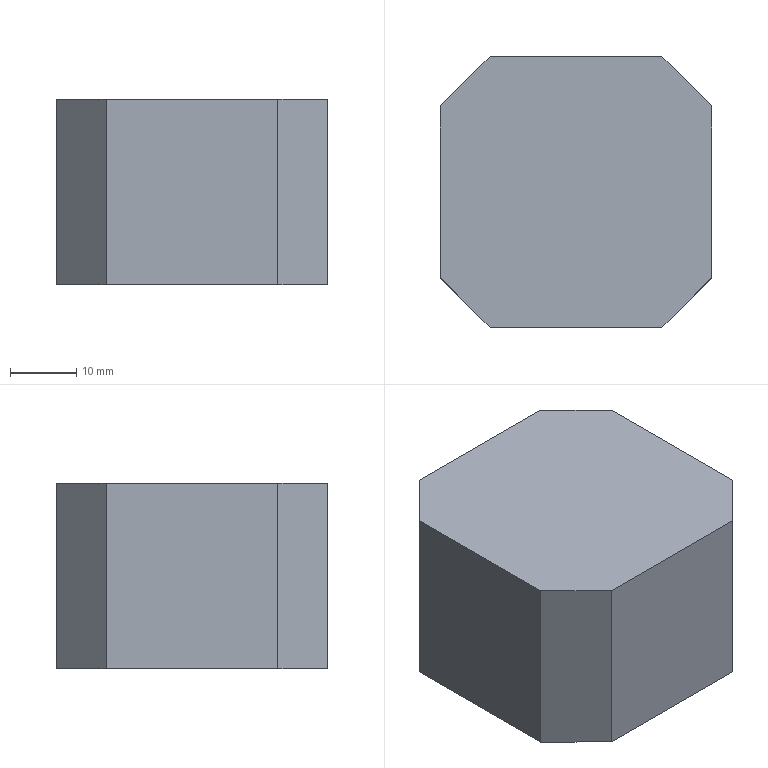Part | SolidWorks | features BaseBody 1 | 1 solid | 10 faces | box 41 x 41 x 28 mm | volume 43918 mm3 | plane 10
STEP:
#1=CARTESIAN_POINT('',(-41.779,25.004,28.));
#2=VERTEX_POINT('',#1);
#3=CARTESIAN_POINT('',(-49.279,17.504,28.));
#4=VERTEX_POINT('',#3);
#5=CARTESIAN_POINT('',(-41.779,25.004,28.));
#6=DIRECTION('',(-0.7071,-0.7071,0.));
#7=VECTOR('',#6,1000.);
#8=LINE('',#5,#7);
#9=EDGE_CURVE('',#2,#4,#8,.T.);
#10=ORIENTED_EDGE('',*,*,#9,.T.);
#11=CARTESIAN_POINT('',(-49.279,-8.496,28.));
#12=VERTEX_POINT('',#11);
#13=CARTESIAN_POINT('',(-49.279,4.504,28.));
#14=DIRECTION('',(0.,-1.,0.));
#15=VECTOR('',#14,1000.);
#16=LINE('',#13,#15);
#17=EDGE_CURVE('',#4,#12,#16,.T.);
#18=ORIENTED_EDGE('',*,*,#17,.T.);
#19=CARTESIAN_POINT('',(-41.779,-15.996,28.));
#20=VERTEX_POINT('',#19);
#21=CARTESIAN_POINT('',(-49.279,-8.496,28.));
#22=DIRECTION('',(0.7071,-0.7071,0.));
#23=VECTOR('',#22,1000.);
#24=LINE('',#21,#23);
#25=EDGE_CURVE('',#12,#20,#24,.T.);
#26=ORIENTED_EDGE('',*,*,#25,.T.);
#27=CARTESIAN_POINT('',(-15.779,-15.996,28.));
#28=VERTEX_POINT('',#27);
#29=CARTESIAN_POINT('',(-28.779,-15.996,28.));
#30=DIRECTION('',(1.,0.,0.));
#31=VECTOR('',#30,1000.);
#32=LINE('',#29,#31);
#33=EDGE_CURVE('',#20,#28,#32,.T.);
#34=ORIENTED_EDGE('',*,*,#33,.T.);
#35=CARTESIAN_POINT('',(-8.279,-8.496,28.));
#36=VERTEX_POINT('',#35);
#37=CARTESIAN_POINT('',(-15.779,-15.996,28.));
#38=DIRECTION('',(0.7071,0.7071,0.));
#39=VECTOR('',#38,1000.);
#40=LINE('',#37,#39);
#41=EDGE_CURVE('',#28,#36,#40,.T.);
#42=ORIENTED_EDGE('',*,*,#41,.T.);
#43=CARTESIAN_POINT('',(-8.279,17.504,28.));
#44=VERTEX_POINT('',#43);
#45=CARTESIAN_POINT('',(-8.279,4.504,28.));
#46=DIRECTION('',(0.,1.,0.));
#47=VECTOR('',#46,1000.);
#48=LINE('',#45,#47);
#49=EDGE_CURVE('',#36,#44,#48,.T.);
#50=ORIENTED_EDGE('',*,*,#49,.T.);
#51=CARTESIAN_POINT('',(-15.779,25.004,28.));
#52=VERTEX_POINT('',#51);
#53=CARTESIAN_POINT('',(-8.279,17.504,28.));
#54=DIRECTION('',(-0.7071,0.7071,0.));
#55=VECTOR('',#54,1000.);
#56=LINE('',#53,#55);
#57=EDGE_CURVE('',#44,#52,#56,.T.);
#58=ORIENTED_EDGE('',*,*,#57,.T.);
#59=CARTESIAN_POINT('',(-28.779,25.004,28.));
#60=DIRECTION('',(-1.,0.,0.));
#61=VECTOR('',#60,1000.);
#62=LINE('',#59,#61);
#63=EDGE_CURVE('',#52,#2,#62,.T.);
#64=ORIENTED_EDGE('',*,*,#63,.T.);
#65=EDGE_LOOP('',(#10,#18,#26,#34,#42,#50,#58,#64));
#66=FACE_OUTER_BOUND('',#65,.T.);
#67=CARTESIAN_POINT('',(-28.779,4.504,28.));
#68=DIRECTION('',(0.,0.,1.));
#69=DIRECTION('',(1.,0.,0.));
#70=AXIS2_PLACEMENT_3D('',#67,#68,#69);
#71=PLANE('',#70);
#72=ADVANCED_FACE('',(#66),#71,.T.);
#73=CARTESIAN_POINT('',(-49.279,17.504,0.));
#74=VERTEX_POINT('',#73);
#75=CARTESIAN_POINT('',(-49.279,17.504,0.));
#76=DIRECTION('',(0.,0.,-1.));
#77=VECTOR('',#76,1000.);
#78=LINE('',#75,#77);
#79=EDGE_CURVE('',#4,#74,#78,.T.);
#80=ORIENTED_EDGE('',*,*,#79,.T.);
#81=CARTESIAN_POINT('',(-49.279,-8.496,0.));
#82=VERTEX_POINT('',#81);
#83=CARTESIAN_POINT('',(-49.279,-15.996,0.));
#84=DIRECTION('',(0.,-1.,0.));
#85=VECTOR('',#84,1000.);
#86=LINE('',#83,#85);
#87=EDGE_CURVE('',#74,#82,#86,.T.);
#88=ORIENTED_EDGE('',*,*,#87,.T.);
#89=CARTESIAN_POINT('',(-49.279,-8.496,0.));
#90=DIRECTION('',(0.,0.,1.));
#91=VECTOR('',#90,1000.);
#92=LINE('',#89,#91);
#93=EDGE_CURVE('',#82,#12,#92,.T.);
#94=ORIENTED_EDGE('',*,*,#93,.T.);
#95=ORIENTED_EDGE('',*,*,#17,.F.);
#96=EDGE_LOOP('',(#80,#88,#94,#95));
#97=FACE_OUTER_BOUND('',#96,.T.);
#98=CARTESIAN_POINT('',(-49.279,-15.996,0.));
#99=DIRECTION('',(-1.,0.,0.));
#100=DIRECTION('',(0.,0.,1.));
#101=AXIS2_PLACEMENT_3D('',#98,#99,#100);
#102=PLANE('',#101);
#103=ADVANCED_FACE('',(#97),#102,.T.);
#104=CARTESIAN_POINT('',(-41.779,25.004,0.));
#105=VERTEX_POINT('',#104);
#106=CARTESIAN_POINT('',(-45.529,21.254,0.));
#107=DIRECTION('',(-0.7071,-0.7071,0.));
#108=VECTOR('',#107,1000.);
#109=LINE('',#106,#108);
#110=EDGE_CURVE('',#105,#74,#109,.T.);
#111=ORIENTED_EDGE('',*,*,#110,.T.);
#112=ORIENTED_EDGE('',*,*,#79,.F.);
#113=ORIENTED_EDGE('',*,*,#9,.F.);
#114=CARTESIAN_POINT('',(-41.779,25.004,0.));
#115=DIRECTION('',(0.,0.,-1.));
#116=VECTOR('',#115,1000.);
#117=LINE('',#114,#116);
#118=EDGE_CURVE('',#2,#105,#117,.T.);
#119=ORIENTED_EDGE('',*,*,#118,.T.);
#120=EDGE_LOOP('',(#111,#112,#113,#119));
#121=FACE_OUTER_BOUND('',#120,.T.);
#122=CARTESIAN_POINT('',(-45.529,21.254,0.));
#123=DIRECTION('',(-0.7071,0.7071,0.));
#124=DIRECTION('',(-0.7071,-0.7071,0.));
#125=AXIS2_PLACEMENT_3D('',#122,#123,#124);
#126=PLANE('',#125);
#127=ADVANCED_FACE('',(#121),#126,.T.);
#128=ORIENTED_EDGE('',*,*,#118,.F.);
#129=ORIENTED_EDGE('',*,*,#63,.F.);
#130=CARTESIAN_POINT('',(-15.779,25.004,0.));
#131=VERTEX_POINT('',#130);
#132=CARTESIAN_POINT('',(-15.779,25.004,0.));
#133=DIRECTION('',(0.,0.,-1.));
#134=VECTOR('',#133,1000.);
#135=LINE('',#132,#134);
#136=EDGE_CURVE('',#52,#131,#135,.T.);
#137=ORIENTED_EDGE('',*,*,#136,.T.);
#138=CARTESIAN_POINT('',(-49.279,25.004,0.));
#139=DIRECTION('',(-1.,0.,0.));
#140=VECTOR('',#139,1000.);
#141=LINE('',#138,#140);
#142=EDGE_CURVE('',#131,#105,#141,.T.);
#143=ORIENTED_EDGE('',*,*,#142,.T.);
#144=EDGE_LOOP('',(#128,#129,#137,#143));
#145=FACE_OUTER_BOUND('',#144,.T.);
#146=CARTESIAN_POINT('',(-49.279,25.004,0.));
#147=DIRECTION('',(0.,1.,0.));
#148=DIRECTION('',(0.,0.,1.));
#149=AXIS2_PLACEMENT_3D('',#146,#147,#148);
#150=PLANE('',#149);
#151=ADVANCED_FACE('',(#145),#150,.T.);
#152=CARTESIAN_POINT('',(-8.279,17.504,0.));
#153=VERTEX_POINT('',#152);
#154=CARTESIAN_POINT('',(-12.029,21.254,0.));
#155=DIRECTION('',(-0.7071,0.7071,0.));
#156=VECTOR('',#155,1000.);
#157=LINE('',#154,#156);
#158=EDGE_CURVE('',#153,#131,#157,.T.);
#159=ORIENTED_EDGE('',*,*,#158,.T.);
#160=ORIENTED_EDGE('',*,*,#136,.F.);
#161=ORIENTED_EDGE('',*,*,#57,.F.);
#162=CARTESIAN_POINT('',(-8.279,17.504,0.));
#163=DIRECTION('',(0.,0.,-1.));
#164=VECTOR('',#163,1000.);
#165=LINE('',#162,#164);
#166=EDGE_CURVE('',#44,#153,#165,.T.);
#167=ORIENTED_EDGE('',*,*,#166,.T.);
#168=EDGE_LOOP('',(#159,#160,#161,#167));
#169=FACE_OUTER_BOUND('',#168,.T.);
#170=CARTESIAN_POINT('',(-12.029,21.254,0.));
#171=DIRECTION('',(0.7071,0.7071,0.));
#172=DIRECTION('',(-0.7071,0.7071,0.));
#173=AXIS2_PLACEMENT_3D('',#170,#171,#172);
#174=PLANE('',#173);
#175=ADVANCED_FACE('',(#169),#174,.T.);
#176=ORIENTED_EDGE('',*,*,#166,.F.);
#177=ORIENTED_EDGE('',*,*,#49,.F.);
#178=CARTESIAN_POINT('',(-8.279,-8.496,0.));
#179=VERTEX_POINT('',#178);
#180=CARTESIAN_POINT('',(-8.279,-8.496,0.));
#181=DIRECTION('',(0.,0.,-1.));
#182=VECTOR('',#181,1000.);
#183=LINE('',#180,#182);
#184=EDGE_CURVE('',#36,#179,#183,.T.);
#185=ORIENTED_EDGE('',*,*,#184,.T.);
#186=CARTESIAN_POINT('',(-8.279,25.004,0.));
#187=DIRECTION('',(0.,1.,0.));
#188=VECTOR('',#187,1000.);
#189=LINE('',#186,#188);
#190=EDGE_CURVE('',#179,#153,#189,.T.);
#191=ORIENTED_EDGE('',*,*,#190,.T.);
#192=EDGE_LOOP('',(#176,#177,#185,#191));
#193=FACE_OUTER_BOUND('',#192,.T.);
#194=CARTESIAN_POINT('',(-8.279,25.004,0.));
#195=DIRECTION('',(1.,0.,0.));
#196=DIRECTION('',(0.,0.,-1.));
#197=AXIS2_PLACEMENT_3D('',#194,#195,#196);
#198=PLANE('',#197);
#199=ADVANCED_FACE('',(#193),#198,.T.);
#200=CARTESIAN_POINT('',(-15.779,-15.996,0.));
#201=VERTEX_POINT('',#200);
#202=CARTESIAN_POINT('',(-12.029,-12.246,0.));
#203=DIRECTION('',(0.7071,0.7071,0.));
#204=VECTOR('',#203,1000.);
#205=LINE('',#202,#204);
#206=EDGE_CURVE('',#201,#179,#205,.T.);
#207=ORIENTED_EDGE('',*,*,#206,.T.);
#208=ORIENTED_EDGE('',*,*,#184,.F.);
#209=ORIENTED_EDGE('',*,*,#41,.F.);
#210=CARTESIAN_POINT('',(-15.779,-15.996,0.));
#211=DIRECTION('',(0.,0.,-1.));
#212=VECTOR('',#211,1000.);
#213=LINE('',#210,#212);
#214=EDGE_CURVE('',#28,#201,#213,.T.);
#215=ORIENTED_EDGE('',*,*,#214,.T.);
#216=EDGE_LOOP('',(#207,#208,#209,#215));
#217=FACE_OUTER_BOUND('',#216,.T.);
#218=CARTESIAN_POINT('',(-12.029,-12.246,0.));
#219=DIRECTION('',(0.7071,-0.7071,0.));
#220=DIRECTION('',(0.7071,0.7071,0.));
#221=AXIS2_PLACEMENT_3D('',#218,#219,#220);
#222=PLANE('',#221);
#223=ADVANCED_FACE('',(#217),#222,.T.);
#224=ORIENTED_EDGE('',*,*,#214,.F.);
#225=ORIENTED_EDGE('',*,*,#33,.F.);
#226=CARTESIAN_POINT('',(-41.779,-15.996,0.));
#227=VERTEX_POINT('',#226);
#228=CARTESIAN_POINT('',(-41.779,-15.996,0.));
#229=DIRECTION('',(0.,0.,-1.));
#230=VECTOR('',#229,1000.);
#231=LINE('',#228,#230);
#232=EDGE_CURVE('',#20,#227,#231,.T.);
#233=ORIENTED_EDGE('',*,*,#232,.T.);
#234=CARTESIAN_POINT('',(-8.279,-15.996,0.));
#235=DIRECTION('',(1.,0.,0.));
#236=VECTOR('',#235,1000.);
#237=LINE('',#234,#236);
#238=EDGE_CURVE('',#227,#201,#237,.T.);
#239=ORIENTED_EDGE('',*,*,#238,.T.);
#240=EDGE_LOOP('',(#224,#225,#233,#239));
#241=FACE_OUTER_BOUND('',#240,.T.);
#242=CARTESIAN_POINT('',(-8.279,-15.996,0.));
#243=DIRECTION('',(0.,-1.,0.));
#244=DIRECTION('',(0.,0.,-1.));
#245=AXIS2_PLACEMENT_3D('',#242,#243,#244);
#246=PLANE('',#245);
#247=ADVANCED_FACE('',(#241),#246,.T.);
#248=CARTESIAN_POINT('',(-45.529,-12.246,0.));
#249=DIRECTION('',(0.7071,-0.7071,0.));
#250=VECTOR('',#249,1000.);
#251=LINE('',#248,#250);
#252=EDGE_CURVE('',#82,#227,#251,.T.);
#253=ORIENTED_EDGE('',*,*,#252,.T.);
#254=ORIENTED_EDGE('',*,*,#232,.F.);
#255=ORIENTED_EDGE('',*,*,#25,.F.);
#256=ORIENTED_EDGE('',*,*,#93,.F.);
#257=EDGE_LOOP('',(#253,#254,#255,#256));
#258=FACE_OUTER_BOUND('',#257,.T.);
#259=CARTESIAN_POINT('',(-45.529,-12.246,0.));
#260=DIRECTION('',(-0.7071,-0.7071,0.));
#261=DIRECTION('',(0.7071,-0.7071,0.));
#262=AXIS2_PLACEMENT_3D('',#259,#260,#261);
#263=PLANE('',#262);
#264=ADVANCED_FACE('',(#258),#263,.T.);
#265=ORIENTED_EDGE('',*,*,#87,.F.);
#266=ORIENTED_EDGE('',*,*,#110,.F.);
#267=ORIENTED_EDGE('',*,*,#142,.F.);
#268=ORIENTED_EDGE('',*,*,#158,.F.);
#269=ORIENTED_EDGE('',*,*,#190,.F.);
#270=ORIENTED_EDGE('',*,*,#206,.F.);
#271=ORIENTED_EDGE('',*,*,#238,.F.);
#272=ORIENTED_EDGE('',*,*,#252,.F.);
#273=EDGE_LOOP('',(#265,#266,#267,#268,#269,#270,#271,#272));
#274=FACE_OUTER_BOUND('',#273,.T.);
#275=CARTESIAN_POINT('',(-28.779,4.504,0.));
#276=DIRECTION('',(0.,0.,1.));
#277=DIRECTION('',(1.,0.,0.));
#278=AXIS2_PLACEMENT_3D('',#275,#276,#277);
#279=PLANE('',#278);
#280=ADVANCED_FACE('',(#274),#279,.F.);
#281=CLOSED_SHELL('',(#72,#103,#127,#151,#175,#199,#223,#247,#264,#280));
#282=MANIFOLD_SOLID_BREP('',#281);
#283=CARTESIAN_POINT('',(0.,0.,0.));
#284=DIRECTION('',(0.,0.,1.));
#285=DIRECTION('',(1.,0.,0.));
#286=AXIS2_PLACEMENT_3D('',#283,#284,#285);
#287=(LENGTH_UNIT()NAMED_UNIT(*)SI_UNIT(.MILLI.,.METRE.));
#288=UNCERTAINTY_MEASURE_WITH_UNIT(LENGTH_MEASURE(0.00001),#287,'','');
#289=(NAMED_UNIT(*)PLANE_ANGLE_UNIT()SI_UNIT($,.RADIAN.));
#290=(NAMED_UNIT(*)SI_UNIT($,.STERADIAN.)SOLID_ANGLE_UNIT());
#291=(GEOMETRIC_REPRESENTATION_CONTEXT(3)GLOBAL_UNCERTAINTY_ASSIGNED_CONTEXT((#288))GLOBAL_UNIT_ASSIGNED_CONTEXT((#287,#289,#290))REPRESENTATION_CONTEXT('',''));
#292=ADVANCED_BREP_SHAPE_REPRESENTATION('',(#282,#286),#291);